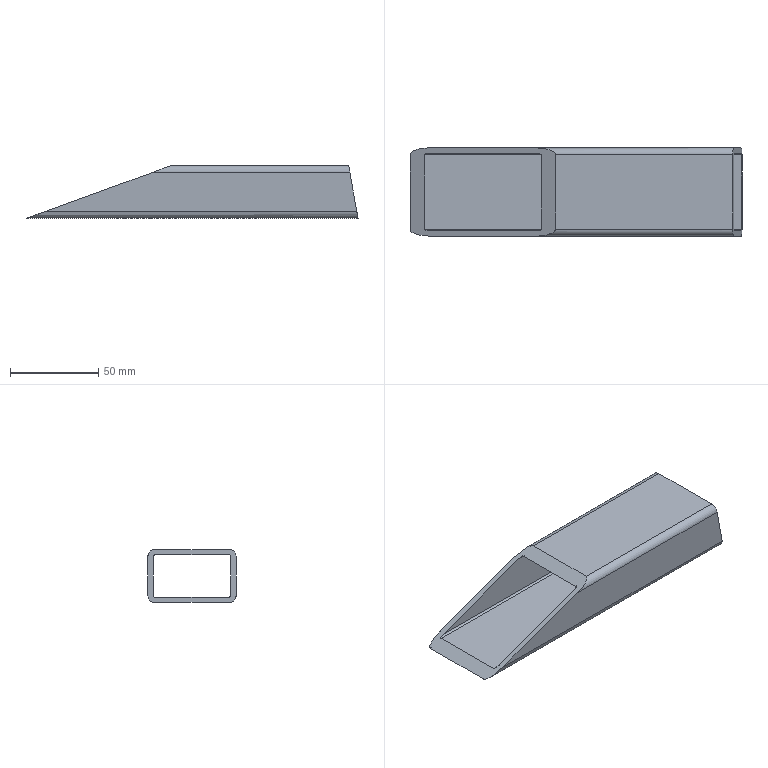Part | SolidWorks | features ICE 2, WeldMemberFeat 1, WeldmentFeature 1 | 1 solid | 18 faces | box 188 x 50 x 30 mm | volume 62143 mm3 | plane 10 | cylinder 8 | commonest cylinder face diameters 2 x4 8 x4
STEP:
#1=CARTESIAN_POINT('',(183.415,25.,11.));
#2=VERTEX_POINT('',#1);
#3=CARTESIAN_POINT('',(71.434,25.,11.));
#4=VERTEX_POINT('',#3);
#5=CARTESIAN_POINT('',(200.,25.,11.));
#6=DIRECTION('',(-1.,0.,0.));
#7=VECTOR('',#6,1000.);
#8=LINE('',#5,#7);
#9=EDGE_CURVE('',#2,#4,#8,.T.);
#10=ORIENTED_EDGE('',*,*,#9,.T.);
#11=CARTESIAN_POINT('',(82.424,21.,15.));
#12=VERTEX_POINT('',#11);
#13=CARTESIAN_POINT('',(71.434,25.,11.));
#14=CARTESIAN_POINT('',(77.872,25.,13.343));
#15=CARTESIAN_POINT('',(82.424,23.343,15.));
#16=CARTESIAN_POINT('',(82.424,21.,15.));
#17=(BOUNDED_CURVE()B_SPLINE_CURVE(3,(#13,#14,#15,#16),.UNSPECIFIED.,.F.,.F.)B_SPLINE_CURVE_WITH_KNOTS((4,4),(1.571,3.142),.UNSPECIFIED.)CURVE()GEOMETRIC_REPRESENTATION_ITEM()RATIONAL_B_SPLINE_CURVE((1.,0.8047,0.8047,1.))REPRESENTATION_ITEM(''));
#18=EDGE_CURVE('',#4,#12,#17,.T.);
#19=ORIENTED_EDGE('',*,*,#18,.T.);
#20=CARTESIAN_POINT('',(182.71,21.,15.));
#21=VERTEX_POINT('',#20);
#22=CARTESIAN_POINT('',(200.,21.,15.));
#23=DIRECTION('',(-1.,0.,0.));
#24=VECTOR('',#23,1000.);
#25=LINE('',#22,#24);
#26=EDGE_CURVE('',#21,#12,#25,.T.);
#27=ORIENTED_EDGE('',*,*,#26,.F.);
#28=CARTESIAN_POINT('',(182.71,21.,15.));
#29=CARTESIAN_POINT('',(182.71,23.343,15.));
#30=CARTESIAN_POINT('',(183.002,25.,13.343));
#31=CARTESIAN_POINT('',(183.415,25.,11.));
#32=(BOUNDED_CURVE()B_SPLINE_CURVE(3,(#28,#29,#30,#31),.UNSPECIFIED.,.F.,.T.)B_SPLINE_CURVE_WITH_KNOTS((4,4),(0.,1.571),.UNSPECIFIED.)CURVE()GEOMETRIC_REPRESENTATION_ITEM()RATIONAL_B_SPLINE_CURVE((1.,0.8047,0.8047,1.))REPRESENTATION_ITEM(''));
#33=EDGE_CURVE('',#21,#2,#32,.T.);
#34=ORIENTED_EDGE('',*,*,#33,.T.);
#35=EDGE_LOOP('',(#10,#19,#27,#34));
#36=FACE_OUTER_BOUND('',#35,.T.);
#37=CARTESIAN_POINT('',(200.,21.,11.));
#38=DIRECTION('',(-1.,0.,0.));
#39=DIRECTION('',(0.,0.,1.));
#40=AXIS2_PLACEMENT_3D('',#37,#38,#39);
#41=CYLINDRICAL_SURFACE('',#40,4.);
#42=ADVANCED_FACE('',(#36),#41,.T.);
#43=ORIENTED_EDGE('',*,*,#26,.T.);
#44=CARTESIAN_POINT('',(82.424,-21.,15.));
#45=VERTEX_POINT('',#44);
#46=CARTESIAN_POINT('',(82.424,-112.,15.));
#47=DIRECTION('',(0.,1.,0.));
#48=VECTOR('',#47,1000.);
#49=LINE('',#46,#48);
#50=EDGE_CURVE('',#45,#12,#49,.T.);
#51=ORIENTED_EDGE('',*,*,#50,.F.);
#52=CARTESIAN_POINT('',(182.71,-21.,15.));
#53=VERTEX_POINT('',#52);
#54=CARTESIAN_POINT('',(200.,-21.,15.));
#55=DIRECTION('',(-1.,0.,0.));
#56=VECTOR('',#55,1000.);
#57=LINE('',#54,#56);
#58=EDGE_CURVE('',#53,#45,#57,.T.);
#59=ORIENTED_EDGE('',*,*,#58,.F.);
#60=CARTESIAN_POINT('',(182.71,-62.,15.));
#61=DIRECTION('',(0.,1.,0.));
#62=VECTOR('',#61,1000.);
#63=LINE('',#60,#62);
#64=EDGE_CURVE('',#53,#21,#63,.T.);
#65=ORIENTED_EDGE('',*,*,#64,.T.);
#66=EDGE_LOOP('',(#43,#51,#59,#65));
#67=FACE_OUTER_BOUND('',#66,.T.);
#68=CARTESIAN_POINT('',(200.,21.,15.));
#69=DIRECTION('',(0.,0.,-1.));
#70=DIRECTION('',(-1.,0.,0.));
#71=AXIS2_PLACEMENT_3D('',#68,#69,#70);
#72=PLANE('',#71);
#73=ADVANCED_FACE('',(#67),#72,.F.);
#74=ORIENTED_EDGE('',*,*,#58,.T.);
#75=CARTESIAN_POINT('',(71.434,-25.,11.));
#76=VERTEX_POINT('',#75);
#77=CARTESIAN_POINT('',(82.424,-21.,15.));
#78=CARTESIAN_POINT('',(82.424,-23.343,15.));
#79=CARTESIAN_POINT('',(77.872,-25.,13.343));
#80=CARTESIAN_POINT('',(71.434,-25.,11.));
#81=(BOUNDED_CURVE()B_SPLINE_CURVE(3,(#77,#78,#79,#80),.UNSPECIFIED.,.F.,.F.)B_SPLINE_CURVE_WITH_KNOTS((4,4),(3.142,4.712),.UNSPECIFIED.)CURVE()GEOMETRIC_REPRESENTATION_ITEM()RATIONAL_B_SPLINE_CURVE((1.,0.8047,0.8047,1.))REPRESENTATION_ITEM(''));
#82=EDGE_CURVE('',#45,#76,#81,.T.);
#83=ORIENTED_EDGE('',*,*,#82,.T.);
#84=CARTESIAN_POINT('',(183.415,-25.,11.));
#85=VERTEX_POINT('',#84);
#86=CARTESIAN_POINT('',(200.,-25.,11.));
#87=DIRECTION('',(-1.,0.,0.));
#88=VECTOR('',#87,1000.);
#89=LINE('',#86,#88);
#90=EDGE_CURVE('',#85,#76,#89,.T.);
#91=ORIENTED_EDGE('',*,*,#90,.F.);
#92=CARTESIAN_POINT('',(183.415,-25.,11.));
#93=CARTESIAN_POINT('',(183.002,-25.,13.343));
#94=CARTESIAN_POINT('',(182.71,-23.343,15.));
#95=CARTESIAN_POINT('',(182.71,-21.,15.));
#96=(BOUNDED_CURVE()B_SPLINE_CURVE(3,(#92,#93,#94,#95),.UNSPECIFIED.,.F.,.F.)B_SPLINE_CURVE_WITH_KNOTS((4,4),(4.712,6.283),.UNSPECIFIED.)CURVE()GEOMETRIC_REPRESENTATION_ITEM()RATIONAL_B_SPLINE_CURVE((1.,0.8047,0.8047,1.))REPRESENTATION_ITEM(''));
#97=EDGE_CURVE('',#85,#53,#96,.T.);
#98=ORIENTED_EDGE('',*,*,#97,.T.);
#99=EDGE_LOOP('',(#74,#83,#91,#98));
#100=FACE_OUTER_BOUND('',#99,.T.);
#101=CARTESIAN_POINT('',(200.,-21.,11.));
#102=DIRECTION('',(-1.,0.,0.));
#103=DIRECTION('',(0.,0.,1.));
#104=AXIS2_PLACEMENT_3D('',#101,#102,#103);
#105=CYLINDRICAL_SURFACE('',#104,4.);
#106=ADVANCED_FACE('',(#100),#105,.T.);
#107=ORIENTED_EDGE('',*,*,#90,.T.);
#108=CARTESIAN_POINT('',(10.99,-25.,-11.));
#109=VERTEX_POINT('',#108);
#110=CARTESIAN_POINT('',(177.89,-25.,49.747));
#111=DIRECTION('',(-0.9397,0.,-0.342));
#112=VECTOR('',#111,1000.);
#113=LINE('',#110,#112);
#114=EDGE_CURVE('',#76,#109,#113,.T.);
#115=ORIENTED_EDGE('',*,*,#114,.T.);
#116=CARTESIAN_POINT('',(187.295,-25.,-11.));
#117=VERTEX_POINT('',#116);
#118=CARTESIAN_POINT('',(200.,-25.,-11.));
#119=DIRECTION('',(-1.,0.,0.));
#120=VECTOR('',#119,1000.);
#121=LINE('',#118,#120);
#122=EDGE_CURVE('',#117,#109,#121,.T.);
#123=ORIENTED_EDGE('',*,*,#122,.F.);
#124=CARTESIAN_POINT('',(187.678,-25.,-13.173));
#125=DIRECTION('',(-0.1736,0.,0.9848));
#126=VECTOR('',#125,1000.);
#127=LINE('',#124,#126);
#128=EDGE_CURVE('',#117,#85,#127,.T.);
#129=ORIENTED_EDGE('',*,*,#128,.T.);
#130=EDGE_LOOP('',(#107,#115,#123,#129));
#131=FACE_OUTER_BOUND('',#130,.T.);
#132=CARTESIAN_POINT('',(200.,-25.,-11.));
#133=DIRECTION('',(0.,1.,0.));
#134=DIRECTION('',(0.,0.,1.));
#135=AXIS2_PLACEMENT_3D('',#132,#133,#134);
#136=PLANE('',#135);
#137=ADVANCED_FACE('',(#131),#136,.F.);
#138=ORIENTED_EDGE('',*,*,#122,.T.);
#139=CARTESIAN_POINT('',(0.,-21.,-15.));
#140=VERTEX_POINT('',#139);
#141=CARTESIAN_POINT('',(10.99,-25.,-11.));
#142=CARTESIAN_POINT('',(4.552,-25.,-13.343));
#143=CARTESIAN_POINT('',(0.,-23.343,-15.));
#144=CARTESIAN_POINT('',(0.,-21.,-15.));
#145=(BOUNDED_CURVE()B_SPLINE_CURVE(3,(#141,#142,#143,#144),.UNSPECIFIED.,.F.,.F.)B_SPLINE_CURVE_WITH_KNOTS((4,4),(4.712,6.283),.UNSPECIFIED.)CURVE()GEOMETRIC_REPRESENTATION_ITEM()RATIONAL_B_SPLINE_CURVE((1.,0.8047,0.8047,1.))REPRESENTATION_ITEM(''));
#146=EDGE_CURVE('',#109,#140,#145,.T.);
#147=ORIENTED_EDGE('',*,*,#146,.T.);
#148=CARTESIAN_POINT('',(188.,-21.,-15.));
#149=VERTEX_POINT('',#148);
#150=CARTESIAN_POINT('',(200.,-21.,-15.));
#151=DIRECTION('',(-1.,0.,0.));
#152=VECTOR('',#151,1000.);
#153=LINE('',#150,#152);
#154=EDGE_CURVE('',#149,#140,#153,.T.);
#155=ORIENTED_EDGE('',*,*,#154,.F.);
#156=CARTESIAN_POINT('',(188.,-21.,-15.));
#157=CARTESIAN_POINT('',(188.,-23.343,-15.));
#158=CARTESIAN_POINT('',(187.708,-25.,-13.343));
#159=CARTESIAN_POINT('',(187.295,-25.,-11.));
#160=(BOUNDED_CURVE()B_SPLINE_CURVE(3,(#156,#157,#158,#159),.UNSPECIFIED.,.F.,.F.)B_SPLINE_CURVE_WITH_KNOTS((4,4),(3.142,4.712),.UNSPECIFIED.)CURVE()GEOMETRIC_REPRESENTATION_ITEM()RATIONAL_B_SPLINE_CURVE((1.,0.8047,0.8047,1.))REPRESENTATION_ITEM(''));
#161=EDGE_CURVE('',#149,#117,#160,.T.);
#162=ORIENTED_EDGE('',*,*,#161,.T.);
#163=EDGE_LOOP('',(#138,#147,#155,#162));
#164=FACE_OUTER_BOUND('',#163,.T.);
#165=CARTESIAN_POINT('',(200.,-21.,-11.));
#166=DIRECTION('',(-1.,0.,0.));
#167=DIRECTION('',(0.,0.,1.));
#168=AXIS2_PLACEMENT_3D('',#165,#166,#167);
#169=CYLINDRICAL_SURFACE('',#168,4.);
#170=ADVANCED_FACE('',(#164),#169,.T.);
#171=CARTESIAN_POINT('',(188.,21.,-15.));
#172=VERTEX_POINT('',#171);
#173=CARTESIAN_POINT('',(0.,21.,-15.));
#174=VERTEX_POINT('',#173);
#175=CARTESIAN_POINT('',(200.,21.,-15.));
#176=DIRECTION('',(-1.,0.,0.));
#177=VECTOR('',#176,1000.);
#178=LINE('',#175,#177);
#179=EDGE_CURVE('',#172,#174,#178,.T.);
#180=ORIENTED_EDGE('',*,*,#179,.F.);
#181=CARTESIAN_POINT('',(188.,-62.,-15.));
#182=DIRECTION('',(0.,1.,0.));
#183=VECTOR('',#182,1000.);
#184=LINE('',#181,#183);
#185=EDGE_CURVE('',#149,#172,#184,.T.);
#186=ORIENTED_EDGE('',*,*,#185,.F.);
#187=ORIENTED_EDGE('',*,*,#154,.T.);
#188=CARTESIAN_POINT('',(0.,-21.,-15.));
#189=DIRECTION('',(0.,1.,0.));
#190=VECTOR('',#189,1000.);
#191=LINE('',#188,#190);
#192=EDGE_CURVE('',#140,#174,#191,.T.);
#193=ORIENTED_EDGE('',*,*,#192,.T.);
#194=EDGE_LOOP('',(#180,#186,#187,#193));
#195=FACE_OUTER_BOUND('',#194,.T.);
#196=CARTESIAN_POINT('',(200.,-21.,-15.));
#197=DIRECTION('',(0.,0.,1.));
#198=DIRECTION('',(1.,0.,0.));
#199=AXIS2_PLACEMENT_3D('',#196,#197,#198);
#200=PLANE('',#199);
#201=ADVANCED_FACE('',(#195),#200,.F.);
#202=ORIENTED_EDGE('',*,*,#179,.T.);
#203=CARTESIAN_POINT('',(10.99,25.,-11.));
#204=VERTEX_POINT('',#203);
#205=CARTESIAN_POINT('',(0.,21.,-15.));
#206=CARTESIAN_POINT('',(0.,23.343,-15.));
#207=CARTESIAN_POINT('',(4.552,25.,-13.343));
#208=CARTESIAN_POINT('',(10.99,25.,-11.));
#209=(BOUNDED_CURVE()B_SPLINE_CURVE(3,(#205,#206,#207,#208),.UNSPECIFIED.,.F.,.F.)B_SPLINE_CURVE_WITH_KNOTS((4,4),(0.,1.571),.UNSPECIFIED.)CURVE()GEOMETRIC_REPRESENTATION_ITEM()RATIONAL_B_SPLINE_CURVE((1.,0.8047,0.8047,1.))REPRESENTATION_ITEM(''));
#210=EDGE_CURVE('',#174,#204,#209,.T.);
#211=ORIENTED_EDGE('',*,*,#210,.T.);
#212=CARTESIAN_POINT('',(187.295,25.,-11.));
#213=VERTEX_POINT('',#212);
#214=CARTESIAN_POINT('',(200.,25.,-11.));
#215=DIRECTION('',(-1.,0.,0.));
#216=VECTOR('',#215,1000.);
#217=LINE('',#214,#216);
#218=EDGE_CURVE('',#213,#204,#217,.T.);
#219=ORIENTED_EDGE('',*,*,#218,.F.);
#220=CARTESIAN_POINT('',(187.295,25.,-11.));
#221=CARTESIAN_POINT('',(187.708,25.,-13.343));
#222=CARTESIAN_POINT('',(188.,23.343,-15.));
#223=CARTESIAN_POINT('',(188.,21.,-15.));
#224=(BOUNDED_CURVE()B_SPLINE_CURVE(3,(#220,#221,#222,#223),.UNSPECIFIED.,.F.,.F.)B_SPLINE_CURVE_WITH_KNOTS((4,4),(1.571,3.142),.UNSPECIFIED.)CURVE()GEOMETRIC_REPRESENTATION_ITEM()RATIONAL_B_SPLINE_CURVE((1.,0.8047,0.8047,1.))REPRESENTATION_ITEM(''));
#225=EDGE_CURVE('',#213,#172,#224,.T.);
#226=ORIENTED_EDGE('',*,*,#225,.T.);
#227=EDGE_LOOP('',(#202,#211,#219,#226));
#228=FACE_OUTER_BOUND('',#227,.T.);
#229=CARTESIAN_POINT('',(200.,21.,-11.));
#230=DIRECTION('',(-1.,0.,0.));
#231=DIRECTION('',(0.,0.,1.));
#232=AXIS2_PLACEMENT_3D('',#229,#230,#231);
#233=CYLINDRICAL_SURFACE('',#232,4.);
#234=ADVANCED_FACE('',(#228),#233,.T.);
#235=CARTESIAN_POINT('',(74.182,-21.,12.));
#236=VERTEX_POINT('',#235);
#237=CARTESIAN_POINT('',(71.434,-22.,11.));
#238=VERTEX_POINT('',#237);
#239=CARTESIAN_POINT('',(74.182,-21.,12.));
#240=CARTESIAN_POINT('',(74.182,-21.586,12.));
#241=CARTESIAN_POINT('',(73.044,-22.,11.586));
#242=CARTESIAN_POINT('',(71.434,-22.,11.));
#243=(BOUNDED_CURVE()B_SPLINE_CURVE(3,(#239,#240,#241,#242),.UNSPECIFIED.,.F.,.F.)B_SPLINE_CURVE_WITH_KNOTS((4,4),(3.142,4.712),.UNSPECIFIED.)CURVE()GEOMETRIC_REPRESENTATION_ITEM()RATIONAL_B_SPLINE_CURVE((1.,0.8047,0.8047,1.))REPRESENTATION_ITEM(''));
#244=EDGE_CURVE('',#236,#238,#243,.T.);
#245=ORIENTED_EDGE('',*,*,#244,.F.);
#246=CARTESIAN_POINT('',(183.239,-21.,12.));
#247=VERTEX_POINT('',#246);
#248=CARTESIAN_POINT('',(200.,-21.,12.));
#249=DIRECTION('',(-1.,0.,0.));
#250=VECTOR('',#249,1000.);
#251=LINE('',#248,#250);
#252=EDGE_CURVE('',#247,#236,#251,.T.);
#253=ORIENTED_EDGE('',*,*,#252,.F.);
#254=CARTESIAN_POINT('',(183.415,-22.,11.));
#255=VERTEX_POINT('',#254);
#256=CARTESIAN_POINT('',(183.415,-22.,11.));
#257=CARTESIAN_POINT('',(183.312,-22.,11.586));
#258=CARTESIAN_POINT('',(183.239,-21.586,12.));
#259=CARTESIAN_POINT('',(183.239,-21.,12.));
#260=(BOUNDED_CURVE()B_SPLINE_CURVE(3,(#256,#257,#258,#259),.UNSPECIFIED.,.F.,.F.)B_SPLINE_CURVE_WITH_KNOTS((4,4),(4.712,6.283),.UNSPECIFIED.)CURVE()GEOMETRIC_REPRESENTATION_ITEM()RATIONAL_B_SPLINE_CURVE((1.,0.8047,0.8047,1.))REPRESENTATION_ITEM(''));
#261=EDGE_CURVE('',#255,#247,#260,.T.);
#262=ORIENTED_EDGE('',*,*,#261,.F.);
#263=CARTESIAN_POINT('',(200.,-22.,11.));
#264=DIRECTION('',(-1.,0.,0.));
#265=VECTOR('',#264,1000.);
#266=LINE('',#263,#265);
#267=EDGE_CURVE('',#255,#238,#266,.T.);
#268=ORIENTED_EDGE('',*,*,#267,.T.);
#269=EDGE_LOOP('',(#245,#253,#262,#268));
#270=FACE_OUTER_BOUND('',#269,.T.);
#271=CARTESIAN_POINT('',(200.,-21.,11.));
#272=DIRECTION('',(-1.,0.,0.));
#273=DIRECTION('',(0.,0.,1.));
#274=AXIS2_PLACEMENT_3D('',#271,#272,#273);
#275=CYLINDRICAL_SURFACE('',#274,1.);
#276=ADVANCED_FACE('',(#270),#275,.F.);
#277=CARTESIAN_POINT('',(74.182,21.,12.));
#278=VERTEX_POINT('',#277);
#279=CARTESIAN_POINT('',(74.182,21.,12.));
#280=DIRECTION('',(0.,-1.,0.));
#281=VECTOR('',#280,1000.);
#282=LINE('',#279,#281);
#283=EDGE_CURVE('',#278,#236,#282,.T.);
#284=ORIENTED_EDGE('',*,*,#283,.F.);
#285=CARTESIAN_POINT('',(183.239,21.,12.));
#286=VERTEX_POINT('',#285);
#287=CARTESIAN_POINT('',(200.,21.,12.));
#288=DIRECTION('',(-1.,0.,0.));
#289=VECTOR('',#288,1000.);
#290=LINE('',#287,#289);
#291=EDGE_CURVE('',#286,#278,#290,.T.);
#292=ORIENTED_EDGE('',*,*,#291,.F.);
#293=CARTESIAN_POINT('',(183.239,21.,12.));
#294=DIRECTION('',(0.,1.,0.));
#295=VECTOR('',#294,1000.);
#296=LINE('',#293,#295);
#297=EDGE_CURVE('',#247,#286,#296,.T.);
#298=ORIENTED_EDGE('',*,*,#297,.F.);
#299=ORIENTED_EDGE('',*,*,#252,.T.);
#300=EDGE_LOOP('',(#284,#292,#298,#299));
#301=FACE_OUTER_BOUND('',#300,.T.);
#302=CARTESIAN_POINT('',(200.,21.,12.));
#303=DIRECTION('',(0.,0.,-1.));
#304=DIRECTION('',(-1.,0.,0.));
#305=AXIS2_PLACEMENT_3D('',#302,#303,#304);
#306=PLANE('',#305);
#307=ADVANCED_FACE('',(#301),#306,.T.);
#308=CARTESIAN_POINT('',(71.434,22.,11.));
#309=VERTEX_POINT('',#308);
#310=CARTESIAN_POINT('',(71.434,22.,11.));
#311=CARTESIAN_POINT('',(73.044,22.,11.586));
#312=CARTESIAN_POINT('',(74.182,21.586,12.));
#313=CARTESIAN_POINT('',(74.182,21.,12.));
#314=(BOUNDED_CURVE()B_SPLINE_CURVE(3,(#310,#311,#312,#313),.UNSPECIFIED.,.F.,.F.)B_SPLINE_CURVE_WITH_KNOTS((4,4),(1.571,3.142),.UNSPECIFIED.)CURVE()GEOMETRIC_REPRESENTATION_ITEM()RATIONAL_B_SPLINE_CURVE((1.,0.8047,0.8047,1.))REPRESENTATION_ITEM(''));
#315=EDGE_CURVE('',#309,#278,#314,.T.);
#316=ORIENTED_EDGE('',*,*,#315,.F.);
#317=CARTESIAN_POINT('',(183.415,22.,11.));
#318=VERTEX_POINT('',#317);
#319=CARTESIAN_POINT('',(200.,22.,11.));
#320=DIRECTION('',(-1.,0.,0.));
#321=VECTOR('',#320,1000.);
#322=LINE('',#319,#321);
#323=EDGE_CURVE('',#318,#309,#322,.T.);
#324=ORIENTED_EDGE('',*,*,#323,.F.);
#325=CARTESIAN_POINT('',(183.239,21.,12.));
#326=CARTESIAN_POINT('',(183.239,21.586,12.));
#327=CARTESIAN_POINT('',(183.312,22.,11.586));
#328=CARTESIAN_POINT('',(183.415,22.,11.));
#329=(BOUNDED_CURVE()B_SPLINE_CURVE(3,(#325,#326,#327,#328),.UNSPECIFIED.,.F.,.F.)B_SPLINE_CURVE_WITH_KNOTS((4,4),(0.,1.571),.UNSPECIFIED.)CURVE()GEOMETRIC_REPRESENTATION_ITEM()RATIONAL_B_SPLINE_CURVE((1.,0.8047,0.8047,1.))REPRESENTATION_ITEM(''));
#330=EDGE_CURVE('',#286,#318,#329,.T.);
#331=ORIENTED_EDGE('',*,*,#330,.F.);
#332=ORIENTED_EDGE('',*,*,#291,.T.);
#333=EDGE_LOOP('',(#316,#324,#331,#332));
#334=FACE_OUTER_BOUND('',#333,.T.);
#335=CARTESIAN_POINT('',(200.,21.,11.));
#336=DIRECTION('',(-1.,0.,0.));
#337=DIRECTION('',(0.,0.,1.));
#338=AXIS2_PLACEMENT_3D('',#335,#336,#337);
#339=CYLINDRICAL_SURFACE('',#338,1.);
#340=ADVANCED_FACE('',(#334),#339,.F.);
#341=CARTESIAN_POINT('',(10.99,22.,-11.));
#342=VERTEX_POINT('',#341);
#343=CARTESIAN_POINT('',(184.961,22.,52.32));
#344=DIRECTION('',(0.9397,0.,0.342));
#345=VECTOR('',#344,1000.);
#346=LINE('',#343,#345);
#347=EDGE_CURVE('',#342,#309,#346,.T.);
#348=ORIENTED_EDGE('',*,*,#347,.F.);
#349=CARTESIAN_POINT('',(187.295,22.,-11.));
#350=VERTEX_POINT('',#349);
#351=CARTESIAN_POINT('',(200.,22.,-11.));
#352=DIRECTION('',(-1.,0.,0.));
#353=VECTOR('',#352,1000.);
#354=LINE('',#351,#353);
#355=EDGE_CURVE('',#350,#342,#354,.T.);
#356=ORIENTED_EDGE('',*,*,#355,.F.);
#357=CARTESIAN_POINT('',(183.916,22.,8.164));
#358=DIRECTION('',(0.1736,0.,-0.9848));
#359=VECTOR('',#358,1000.);
#360=LINE('',#357,#359);
#361=EDGE_CURVE('',#318,#350,#360,.T.);
#362=ORIENTED_EDGE('',*,*,#361,.F.);
#363=ORIENTED_EDGE('',*,*,#323,.T.);
#364=EDGE_LOOP('',(#348,#356,#362,#363));
#365=FACE_OUTER_BOUND('',#364,.T.);
#366=CARTESIAN_POINT('',(200.,22.,11.));
#367=DIRECTION('',(0.,-1.,0.));
#368=DIRECTION('',(0.,0.,-1.));
#369=AXIS2_PLACEMENT_3D('',#366,#367,#368);
#370=PLANE('',#369);
#371=ADVANCED_FACE('',(#365),#370,.T.);
#372=CARTESIAN_POINT('',(8.242,21.,-12.));
#373=VERTEX_POINT('',#372);
#374=CARTESIAN_POINT('',(8.242,21.,-12.));
#375=CARTESIAN_POINT('',(8.242,21.586,-12.));
#376=CARTESIAN_POINT('',(9.38,22.,-11.586));
#377=CARTESIAN_POINT('',(10.99,22.,-11.));
#378=(BOUNDED_CURVE()B_SPLINE_CURVE(3,(#374,#375,#376,#377),.UNSPECIFIED.,.F.,.T.)B_SPLINE_CURVE_WITH_KNOTS((4,4),(0.,1.571),.UNSPECIFIED.)CURVE()GEOMETRIC_REPRESENTATION_ITEM()RATIONAL_B_SPLINE_CURVE((1.,0.8047,0.8047,1.))REPRESENTATION_ITEM(''));
#379=EDGE_CURVE('',#373,#342,#378,.T.);
#380=ORIENTED_EDGE('',*,*,#379,.F.);
#381=CARTESIAN_POINT('',(187.471,21.,-12.));
#382=VERTEX_POINT('',#381);
#383=CARTESIAN_POINT('',(200.,21.,-12.));
#384=DIRECTION('',(-1.,0.,0.));
#385=VECTOR('',#384,1000.);
#386=LINE('',#383,#385);
#387=EDGE_CURVE('',#382,#373,#386,.T.);
#388=ORIENTED_EDGE('',*,*,#387,.F.);
#389=CARTESIAN_POINT('',(187.295,22.,-11.));
#390=CARTESIAN_POINT('',(187.398,22.,-11.586));
#391=CARTESIAN_POINT('',(187.471,21.586,-12.));
#392=CARTESIAN_POINT('',(187.471,21.,-12.));
#393=(BOUNDED_CURVE()B_SPLINE_CURVE(3,(#389,#390,#391,#392),.UNSPECIFIED.,.F.,.F.)B_SPLINE_CURVE_WITH_KNOTS((4,4),(1.571,3.142),.UNSPECIFIED.)CURVE()GEOMETRIC_REPRESENTATION_ITEM()RATIONAL_B_SPLINE_CURVE((1.,0.8047,0.8047,1.))REPRESENTATION_ITEM(''));
#394=EDGE_CURVE('',#350,#382,#393,.T.);
#395=ORIENTED_EDGE('',*,*,#394,.F.);
#396=ORIENTED_EDGE('',*,*,#355,.T.);
#397=EDGE_LOOP('',(#380,#388,#395,#396));
#398=FACE_OUTER_BOUND('',#397,.T.);
#399=CARTESIAN_POINT('',(200.,21.,-11.));
#400=DIRECTION('',(-1.,0.,0.));
#401=DIRECTION('',(0.,0.,1.));
#402=AXIS2_PLACEMENT_3D('',#399,#400,#401);
#403=CYLINDRICAL_SURFACE('',#402,1.);
#404=ADVANCED_FACE('',(#398),#403,.F.);
#405=CARTESIAN_POINT('',(8.242,-21.,-12.));
#406=VERTEX_POINT('',#405);
#407=CARTESIAN_POINT('',(8.242,-21.,-12.));
#408=DIRECTION('',(0.,1.,0.));
#409=VECTOR('',#408,1000.);
#410=LINE('',#407,#409);
#411=EDGE_CURVE('',#406,#373,#410,.T.);
#412=ORIENTED_EDGE('',*,*,#411,.F.);
#413=CARTESIAN_POINT('',(187.471,-21.,-12.));
#414=VERTEX_POINT('',#413);
#415=CARTESIAN_POINT('',(200.,-21.,-12.));
#416=DIRECTION('',(-1.,0.,0.));
#417=VECTOR('',#416,1000.);
#418=LINE('',#415,#417);
#419=EDGE_CURVE('',#414,#406,#418,.T.);
#420=ORIENTED_EDGE('',*,*,#419,.F.);
#421=CARTESIAN_POINT('',(187.471,-21.,-12.));
#422=DIRECTION('',(0.,-1.,0.));
#423=VECTOR('',#422,1000.);
#424=LINE('',#421,#423);
#425=EDGE_CURVE('',#382,#414,#424,.T.);
#426=ORIENTED_EDGE('',*,*,#425,.F.);
#427=ORIENTED_EDGE('',*,*,#387,.T.);
#428=EDGE_LOOP('',(#412,#420,#426,#427));
#429=FACE_OUTER_BOUND('',#428,.T.);
#430=CARTESIAN_POINT('',(200.,-21.,-12.));
#431=DIRECTION('',(0.,0.,1.));
#432=DIRECTION('',(1.,0.,0.));
#433=AXIS2_PLACEMENT_3D('',#430,#431,#432);
#434=PLANE('',#433);
#435=ADVANCED_FACE('',(#429),#434,.T.);
#436=CARTESIAN_POINT('',(10.99,-22.,-11.));
#437=VERTEX_POINT('',#436);
#438=CARTESIAN_POINT('',(10.99,-22.,-11.));
#439=CARTESIAN_POINT('',(9.38,-22.,-11.586));
#440=CARTESIAN_POINT('',(8.242,-21.586,-12.));
#441=CARTESIAN_POINT('',(8.242,-21.,-12.));
#442=(BOUNDED_CURVE()B_SPLINE_CURVE(3,(#438,#439,#440,#441),.UNSPECIFIED.,.F.,.F.)B_SPLINE_CURVE_WITH_KNOTS((4,4),(4.712,6.283),.UNSPECIFIED.)CURVE()GEOMETRIC_REPRESENTATION_ITEM()RATIONAL_B_SPLINE_CURVE((1.,0.8047,0.8047,1.))REPRESENTATION_ITEM(''));
#443=EDGE_CURVE('',#437,#406,#442,.T.);
#444=ORIENTED_EDGE('',*,*,#443,.F.);
#445=CARTESIAN_POINT('',(187.295,-22.,-11.));
#446=VERTEX_POINT('',#445);
#447=CARTESIAN_POINT('',(200.,-22.,-11.));
#448=DIRECTION('',(-1.,0.,0.));
#449=VECTOR('',#448,1000.);
#450=LINE('',#447,#449);
#451=EDGE_CURVE('',#446,#437,#450,.T.);
#452=ORIENTED_EDGE('',*,*,#451,.F.);
#453=CARTESIAN_POINT('',(187.471,-21.,-12.));
#454=CARTESIAN_POINT('',(187.471,-21.586,-12.));
#455=CARTESIAN_POINT('',(187.398,-22.,-11.586));
#456=CARTESIAN_POINT('',(187.295,-22.,-11.));
#457=(BOUNDED_CURVE()B_SPLINE_CURVE(3,(#453,#454,#455,#456),.UNSPECIFIED.,.F.,.F.)B_SPLINE_CURVE_WITH_KNOTS((4,4),(3.142,4.712),.UNSPECIFIED.)CURVE()GEOMETRIC_REPRESENTATION_ITEM()RATIONAL_B_SPLINE_CURVE((1.,0.8047,0.8047,1.))REPRESENTATION_ITEM(''));
#458=EDGE_CURVE('',#414,#446,#457,.T.);
#459=ORIENTED_EDGE('',*,*,#458,.F.);
#460=ORIENTED_EDGE('',*,*,#419,.T.);
#461=EDGE_LOOP('',(#444,#452,#459,#460));
#462=FACE_OUTER_BOUND('',#461,.T.);
#463=CARTESIAN_POINT('',(200.,-21.,-11.));
#464=DIRECTION('',(-1.,0.,0.));
#465=DIRECTION('',(0.,0.,1.));
#466=AXIS2_PLACEMENT_3D('',#463,#464,#465);
#467=CYLINDRICAL_SURFACE('',#466,1.);
#468=ADVANCED_FACE('',(#462),#467,.F.);
#469=CARTESIAN_POINT('',(177.89,-22.,49.747));
#470=DIRECTION('',(-0.9397,0.,-0.342));
#471=VECTOR('',#470,1000.);
#472=LINE('',#469,#471);
#473=EDGE_CURVE('',#238,#437,#472,.T.);
#474=ORIENTED_EDGE('',*,*,#473,.F.);
#475=ORIENTED_EDGE('',*,*,#267,.F.);
#476=CARTESIAN_POINT('',(187.678,-22.,-13.173));
#477=DIRECTION('',(-0.1736,0.,0.9848));
#478=VECTOR('',#477,1000.);
#479=LINE('',#476,#478);
#480=EDGE_CURVE('',#446,#255,#479,.T.);
#481=ORIENTED_EDGE('',*,*,#480,.F.);
#482=ORIENTED_EDGE('',*,*,#451,.T.);
#483=EDGE_LOOP('',(#474,#475,#481,#482));
#484=FACE_OUTER_BOUND('',#483,.T.);
#485=CARTESIAN_POINT('',(200.,-22.,-11.));
#486=DIRECTION('',(0.,1.,0.));
#487=DIRECTION('',(0.,0.,1.));
#488=AXIS2_PLACEMENT_3D('',#485,#486,#487);
#489=PLANE('',#488);
#490=ADVANCED_FACE('',(#484),#489,.T.);
#491=ORIENTED_EDGE('',*,*,#218,.T.);
#492=CARTESIAN_POINT('',(0.,25.,-15.));
#493=DIRECTION('',(-0.9397,0.,-0.342));
#494=VECTOR('',#493,1000.);
#495=LINE('',#492,#494);
#496=EDGE_CURVE('',#4,#204,#495,.T.);
#497=ORIENTED_EDGE('',*,*,#496,.F.);
#498=ORIENTED_EDGE('',*,*,#9,.F.);
#499=CARTESIAN_POINT('',(188.,25.,-15.));
#500=DIRECTION('',(-0.1736,0.,0.9848));
#501=VECTOR('',#500,1000.);
#502=LINE('',#499,#501);
#503=EDGE_CURVE('',#213,#2,#502,.T.);
#504=ORIENTED_EDGE('',*,*,#503,.F.);
#505=EDGE_LOOP('',(#491,#497,#498,#504));
#506=FACE_OUTER_BOUND('',#505,.T.);
#507=CARTESIAN_POINT('',(200.,25.,11.));
#508=DIRECTION('',(0.,-1.,0.));
#509=DIRECTION('',(0.,0.,-1.));
#510=AXIS2_PLACEMENT_3D('',#507,#508,#509);
#511=PLANE('',#510);
#512=ADVANCED_FACE('',(#506),#511,.F.);
#513=ORIENTED_EDGE('',*,*,#261,.T.);
#514=ORIENTED_EDGE('',*,*,#297,.T.);
#515=ORIENTED_EDGE('',*,*,#330,.T.);
#516=ORIENTED_EDGE('',*,*,#361,.T.);
#517=ORIENTED_EDGE('',*,*,#394,.T.);
#518=ORIENTED_EDGE('',*,*,#425,.T.);
#519=ORIENTED_EDGE('',*,*,#458,.T.);
#520=ORIENTED_EDGE('',*,*,#480,.T.);
#521=EDGE_LOOP('',(#513,#514,#515,#516,#517,#518,#519,#520));
#522=FACE_BOUND('',#521,.T.);
#523=ORIENTED_EDGE('',*,*,#64,.F.);
#524=ORIENTED_EDGE('',*,*,#97,.F.);
#525=ORIENTED_EDGE('',*,*,#128,.F.);
#526=ORIENTED_EDGE('',*,*,#161,.F.);
#527=ORIENTED_EDGE('',*,*,#185,.T.);
#528=ORIENTED_EDGE('',*,*,#225,.F.);
#529=ORIENTED_EDGE('',*,*,#503,.T.);
#530=ORIENTED_EDGE('',*,*,#33,.F.);
#531=EDGE_LOOP('',(#523,#524,#525,#526,#527,#528,#529,#530));
#532=FACE_OUTER_BOUND('',#531,.T.);
#533=CARTESIAN_POINT('',(188.,-62.,-15.));
#534=DIRECTION('',(-0.9848,0.,-0.1736));
#535=DIRECTION('',(-0.1736,0.,0.9848));
#536=AXIS2_PLACEMENT_3D('',#533,#534,#535);
#537=PLANE('',#536);
#538=ADVANCED_FACE('',(#522,#532),#537,.F.);
#539=ORIENTED_EDGE('',*,*,#244,.T.);
#540=ORIENTED_EDGE('',*,*,#473,.T.);
#541=ORIENTED_EDGE('',*,*,#443,.T.);
#542=ORIENTED_EDGE('',*,*,#411,.T.);
#543=ORIENTED_EDGE('',*,*,#379,.T.);
#544=ORIENTED_EDGE('',*,*,#347,.T.);
#545=ORIENTED_EDGE('',*,*,#315,.T.);
#546=ORIENTED_EDGE('',*,*,#283,.T.);
#547=EDGE_LOOP('',(#539,#540,#541,#542,#543,#544,#545,#546));
#548=FACE_BOUND('',#547,.T.);
#549=ORIENTED_EDGE('',*,*,#496,.T.);
#550=ORIENTED_EDGE('',*,*,#210,.F.);
#551=ORIENTED_EDGE('',*,*,#192,.F.);
#552=ORIENTED_EDGE('',*,*,#146,.F.);
#553=ORIENTED_EDGE('',*,*,#114,.F.);
#554=ORIENTED_EDGE('',*,*,#82,.F.);
#555=ORIENTED_EDGE('',*,*,#50,.T.);
#556=ORIENTED_EDGE('',*,*,#18,.F.);
#557=EDGE_LOOP('',(#549,#550,#551,#552,#553,#554,#555,#556));
#558=FACE_OUTER_BOUND('',#557,.T.);
#559=CARTESIAN_POINT('',(0.,-112.,-15.));
#560=DIRECTION('',(0.342,0.,-0.9397));
#561=DIRECTION('',(-0.9397,0.,-0.342));
#562=AXIS2_PLACEMENT_3D('',#559,#560,#561);
#563=PLANE('',#562);
#564=ADVANCED_FACE('',(#548,#558),#563,.F.);
#565=CLOSED_SHELL('',(#42,#73,#106,#137,#170,#201,#234,#276,#307,#340,#371,#404,#435,#468,#490,#512,#538,#564));
#566=MANIFOLD_SOLID_BREP('',#565);
#567=CARTESIAN_POINT('',(0.,0.,0.));
#568=DIRECTION('',(0.,0.,1.));
#569=DIRECTION('',(1.,0.,0.));
#570=AXIS2_PLACEMENT_3D('',#567,#568,#569);
#571=(LENGTH_UNIT()NAMED_UNIT(*)SI_UNIT(.MILLI.,.METRE.));
#572=UNCERTAINTY_MEASURE_WITH_UNIT(LENGTH_MEASURE(0.00001),#571,'','');
#573=(NAMED_UNIT(*)PLANE_ANGLE_UNIT()SI_UNIT($,.RADIAN.));
#574=(NAMED_UNIT(*)SI_UNIT($,.STERADIAN.)SOLID_ANGLE_UNIT());
#575=(GEOMETRIC_REPRESENTATION_CONTEXT(3)GLOBAL_UNCERTAINTY_ASSIGNED_CONTEXT((#572))GLOBAL_UNIT_ASSIGNED_CONTEXT((#571,#573,#574))REPRESENTATION_CONTEXT('',''));
#576=ADVANCED_BREP_SHAPE_REPRESENTATION('',(#566,#570),#575);